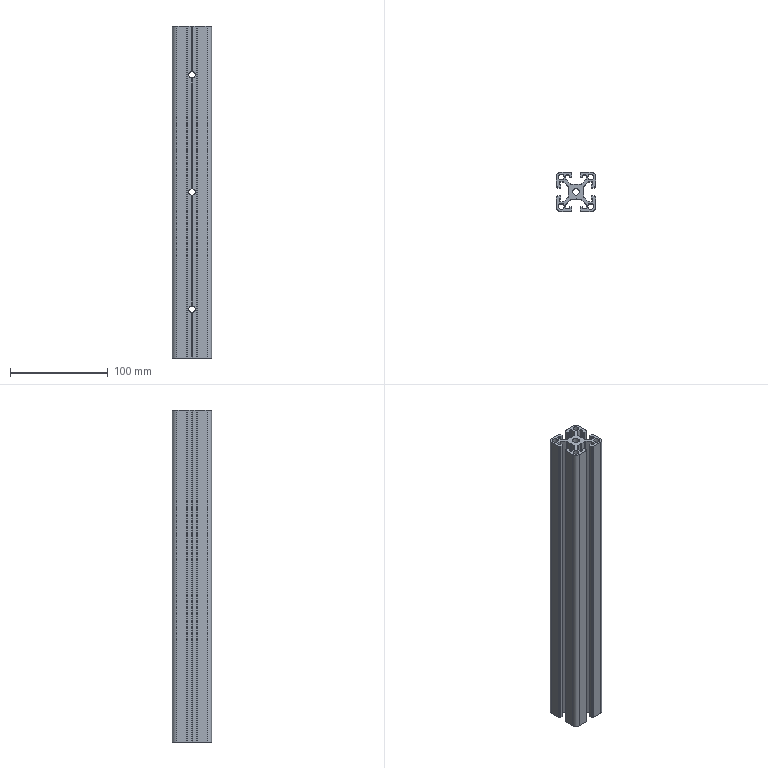Part | STEP file | HM-8-4040D-L340-machining required | 1 solid | 248 faces | box 40 x 40 x 340 mm | volume 231664 mm3 | cylinder 128 | plane 120 | commonest cylinder face diameters 1 x46 0.4 x42 6.6 x12 4 x8 6 x8 11 x6